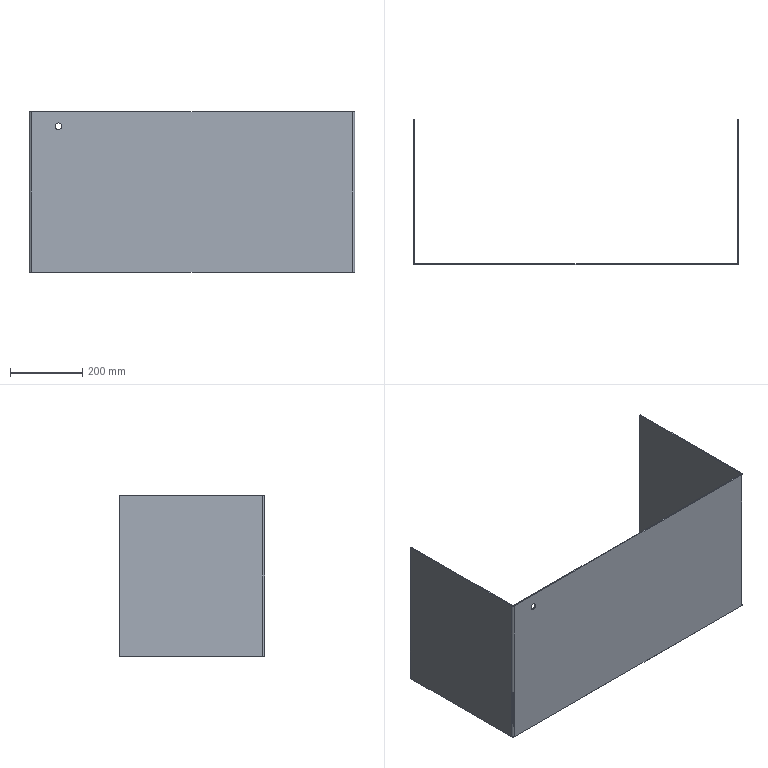Part | SolidWorks | features ICE 2, FlatPattern 1, SMBaseFlange 1, SheetMetal 1 | 1 solid | 28 faces | box 900 x 403 x 444 mm | volume 2258443 mm3 | plane 18 | cylinder 10 | commonest cylinder face diameters 7 x4 6 x2 12 x2 18.2 x2
STEP:
#1=CARTESIAN_POINT('',(80.,-403.,394.9));
#2=VERTEX_POINT('',#1);
#3=CARTESIAN_POINT('',(80.,-403.,413.1));
#4=VERTEX_POINT('',#3);
#5=CARTESIAN_POINT('',(80.,-403.,404.));
#6=DIRECTION('',(0.,1.,0.));
#7=DIRECTION('',(0.,0.,1.));
#8=AXIS2_PLACEMENT_3D('',#5,#6,#7);
#9=CIRCLE('',#8,9.1);
#10=EDGE_CURVE('',#2,#4,#9,.T.);
#11=ORIENTED_EDGE('',*,*,#10,.F.);
#12=CARTESIAN_POINT('',(80.,-400.,394.9));
#13=VERTEX_POINT('',#12);
#14=CARTESIAN_POINT('',(80.,-410.,394.9));
#15=DIRECTION('',(0.,1.,0.));
#16=VECTOR('',#15,1000.);
#17=LINE('',#14,#16);
#18=EDGE_CURVE('',#2,#13,#17,.T.);
#19=ORIENTED_EDGE('',*,*,#18,.T.);
#20=CARTESIAN_POINT('',(80.,-400.,413.1));
#21=VERTEX_POINT('',#20);
#22=CARTESIAN_POINT('',(80.,-400.,404.));
#23=DIRECTION('',(0.,1.,0.));
#24=DIRECTION('',(0.,0.,1.));
#25=AXIS2_PLACEMENT_3D('',#22,#23,#24);
#26=CIRCLE('',#25,9.1);
#27=EDGE_CURVE('',#13,#21,#26,.T.);
#28=ORIENTED_EDGE('',*,*,#27,.T.);
#29=CARTESIAN_POINT('',(80.,-410.,413.1));
#30=DIRECTION('',(0.,1.,0.));
#31=VECTOR('',#30,1000.);
#32=LINE('',#29,#31);
#33=EDGE_CURVE('',#4,#21,#32,.T.);
#34=ORIENTED_EDGE('',*,*,#33,.F.);
#35=EDGE_LOOP('',(#11,#19,#28,#34));
#36=FACE_OUTER_BOUND('',#35,.T.);
#37=CARTESIAN_POINT('',(80.,-410.,404.));
#38=DIRECTION('',(0.,1.,0.));
#39=DIRECTION('',(0.,0.,1.));
#40=AXIS2_PLACEMENT_3D('',#37,#38,#39);
#41=CYLINDRICAL_SURFACE('',#40,9.1);
#42=ADVANCED_FACE('',(#36),#41,.F.);
#43=CARTESIAN_POINT('',(900.,-3.5,0.));
#44=VERTEX_POINT('',#43);
#45=CARTESIAN_POINT('',(900.,0.,3.5));
#46=VERTEX_POINT('',#45);
#47=CARTESIAN_POINT('',(900.,-3.5,3.5));
#48=DIRECTION('',(1.,0.,0.));
#49=DIRECTION('',(0.,0.,1.));
#50=AXIS2_PLACEMENT_3D('',#47,#48,#49);
#51=CIRCLE('',#50,3.5);
#52=EDGE_CURVE('',#44,#46,#51,.T.);
#53=ORIENTED_EDGE('',*,*,#52,.T.);
#54=CARTESIAN_POINT('',(900.,0.,440.5));
#55=VERTEX_POINT('',#54);
#56=CARTESIAN_POINT('',(900.,0.,444.));
#57=DIRECTION('',(0.,0.,-1.));
#58=VECTOR('',#57,1000.);
#59=LINE('',#56,#58);
#60=EDGE_CURVE('',#55,#46,#59,.T.);
#61=ORIENTED_EDGE('',*,*,#60,.F.);
#62=CARTESIAN_POINT('',(900.,-3.5,444.));
#63=VERTEX_POINT('',#62);
#64=CARTESIAN_POINT('',(900.,-3.5,440.5));
#65=DIRECTION('',(1.,0.,0.));
#66=DIRECTION('',(0.,0.,1.));
#67=AXIS2_PLACEMENT_3D('',#64,#65,#66);
#68=CIRCLE('',#67,3.5);
#69=EDGE_CURVE('',#55,#63,#68,.T.);
#70=ORIENTED_EDGE('',*,*,#69,.T.);
#71=CARTESIAN_POINT('',(900.,-397.,444.));
#72=VERTEX_POINT('',#71);
#73=CARTESIAN_POINT('',(900.,-403.,444.));
#74=DIRECTION('',(0.,1.,0.));
#75=VECTOR('',#74,1000.);
#76=LINE('',#73,#75);
#77=EDGE_CURVE('',#72,#63,#76,.T.);
#78=ORIENTED_EDGE('',*,*,#77,.F.);
#79=CARTESIAN_POINT('',(900.,-397.,0.));
#80=VERTEX_POINT('',#79);
#81=CARTESIAN_POINT('',(900.,-397.,444.));
#82=DIRECTION('',(0.,0.,-1.));
#83=VECTOR('',#82,1000.);
#84=LINE('',#81,#83);
#85=EDGE_CURVE('',#72,#80,#84,.T.);
#86=ORIENTED_EDGE('',*,*,#85,.T.);
#87=CARTESIAN_POINT('',(900.,-403.,0.));
#88=DIRECTION('',(0.,1.,0.));
#89=VECTOR('',#88,1000.);
#90=LINE('',#87,#89);
#91=EDGE_CURVE('',#80,#44,#90,.T.);
#92=ORIENTED_EDGE('',*,*,#91,.T.);
#93=EDGE_LOOP('',(#53,#61,#70,#78,#86,#92));
#94=FACE_OUTER_BOUND('',#93,.T.);
#95=CARTESIAN_POINT('',(900.,-403.,444.));
#96=DIRECTION('',(-1.,0.,0.));
#97=DIRECTION('',(0.,0.,1.));
#98=AXIS2_PLACEMENT_3D('',#95,#96,#97);
#99=PLANE('',#98);
#100=ADVANCED_FACE('',(#94),#99,.F.);
#101=CARTESIAN_POINT('',(897.,0.,440.5));
#102=VERTEX_POINT('',#101);
#103=CARTESIAN_POINT('',(897.,0.,3.5));
#104=VERTEX_POINT('',#103);
#105=CARTESIAN_POINT('',(897.,0.,444.));
#106=DIRECTION('',(0.,0.,-1.));
#107=VECTOR('',#106,1000.);
#108=LINE('',#105,#107);
#109=EDGE_CURVE('',#102,#104,#108,.T.);
#110=ORIENTED_EDGE('',*,*,#109,.T.);
#111=CARTESIAN_POINT('',(897.,-3.5,0.));
#112=VERTEX_POINT('',#111);
#113=CARTESIAN_POINT('',(897.,-3.5,3.5));
#114=DIRECTION('',(1.,0.,0.));
#115=DIRECTION('',(0.,0.,1.));
#116=AXIS2_PLACEMENT_3D('',#113,#114,#115);
#117=CIRCLE('',#116,3.5);
#118=EDGE_CURVE('',#112,#104,#117,.T.);
#119=ORIENTED_EDGE('',*,*,#118,.F.);
#120=CARTESIAN_POINT('',(897.,-397.,0.));
#121=VERTEX_POINT('',#120);
#122=CARTESIAN_POINT('',(897.,-403.,0.));
#123=DIRECTION('',(0.,1.,0.));
#124=VECTOR('',#123,1000.);
#125=LINE('',#122,#124);
#126=EDGE_CURVE('',#121,#112,#125,.T.);
#127=ORIENTED_EDGE('',*,*,#126,.F.);
#128=CARTESIAN_POINT('',(897.,-397.,444.));
#129=VERTEX_POINT('',#128);
#130=CARTESIAN_POINT('',(897.,-397.,444.));
#131=DIRECTION('',(0.,0.,-1.));
#132=VECTOR('',#131,1000.);
#133=LINE('',#130,#132);
#134=EDGE_CURVE('',#129,#121,#133,.T.);
#135=ORIENTED_EDGE('',*,*,#134,.F.);
#136=CARTESIAN_POINT('',(897.,-3.5,444.));
#137=VERTEX_POINT('',#136);
#138=CARTESIAN_POINT('',(897.,-403.,444.));
#139=DIRECTION('',(0.,1.,0.));
#140=VECTOR('',#139,1000.);
#141=LINE('',#138,#140);
#142=EDGE_CURVE('',#129,#137,#141,.T.);
#143=ORIENTED_EDGE('',*,*,#142,.T.);
#144=CARTESIAN_POINT('',(897.,-3.5,440.5));
#145=DIRECTION('',(1.,0.,0.));
#146=DIRECTION('',(0.,0.,1.));
#147=AXIS2_PLACEMENT_3D('',#144,#145,#146);
#148=CIRCLE('',#147,3.5);
#149=EDGE_CURVE('',#102,#137,#148,.T.);
#150=ORIENTED_EDGE('',*,*,#149,.F.);
#151=EDGE_LOOP('',(#110,#119,#127,#135,#143,#150));
#152=FACE_OUTER_BOUND('',#151,.T.);
#153=CARTESIAN_POINT('',(897.,-403.,444.));
#154=DIRECTION('',(-1.,0.,0.));
#155=DIRECTION('',(0.,0.,1.));
#156=AXIS2_PLACEMENT_3D('',#153,#154,#155);
#157=PLANE('',#156);
#158=ADVANCED_FACE('',(#152),#157,.T.);
#159=ORIENTED_EDGE('',*,*,#60,.T.);
#160=CARTESIAN_POINT('',(897.,0.,3.5));
#161=DIRECTION('',(1.,0.,0.));
#162=VECTOR('',#161,1000.);
#163=LINE('',#160,#162);
#164=EDGE_CURVE('',#104,#46,#163,.T.);
#165=ORIENTED_EDGE('',*,*,#164,.F.);
#166=ORIENTED_EDGE('',*,*,#109,.F.);
#167=CARTESIAN_POINT('',(897.,0.,440.5));
#168=DIRECTION('',(1.,0.,0.));
#169=VECTOR('',#168,1000.);
#170=LINE('',#167,#169);
#171=EDGE_CURVE('',#102,#55,#170,.T.);
#172=ORIENTED_EDGE('',*,*,#171,.T.);
#173=EDGE_LOOP('',(#159,#165,#166,#172));
#174=FACE_OUTER_BOUND('',#173,.T.);
#175=CARTESIAN_POINT('',(897.,0.,444.));
#176=DIRECTION('',(0.,1.,0.));
#177=DIRECTION('',(0.,0.,1.));
#178=AXIS2_PLACEMENT_3D('',#175,#176,#177);
#179=PLANE('',#178);
#180=ADVANCED_FACE('',(#174),#179,.T.);
#181=CARTESIAN_POINT('',(3.,-3.5,0.));
#182=VERTEX_POINT('',#181);
#183=CARTESIAN_POINT('',(3.,-397.,0.));
#184=VERTEX_POINT('',#183);
#185=CARTESIAN_POINT('',(3.,0.,0.));
#186=DIRECTION('',(0.,-1.,0.));
#187=VECTOR('',#186,1000.);
#188=LINE('',#185,#187);
#189=EDGE_CURVE('',#182,#184,#188,.T.);
#190=ORIENTED_EDGE('',*,*,#189,.F.);
#191=CARTESIAN_POINT('',(3.,0.,3.5));
#192=VERTEX_POINT('',#191);
#193=CARTESIAN_POINT('',(3.,-3.5,3.5));
#194=DIRECTION('',(-1.,0.,0.));
#195=DIRECTION('',(0.,1.,0.));
#196=AXIS2_PLACEMENT_3D('',#193,#194,#195);
#197=CIRCLE('',#196,3.5);
#198=EDGE_CURVE('',#192,#182,#197,.T.);
#199=ORIENTED_EDGE('',*,*,#198,.F.);
#200=CARTESIAN_POINT('',(3.,0.,440.5));
#201=VERTEX_POINT('',#200);
#202=CARTESIAN_POINT('',(3.,0.,444.));
#203=DIRECTION('',(0.,0.,-1.));
#204=VECTOR('',#203,1000.);
#205=LINE('',#202,#204);
#206=EDGE_CURVE('',#201,#192,#205,.T.);
#207=ORIENTED_EDGE('',*,*,#206,.F.);
#208=CARTESIAN_POINT('',(3.,-3.5,444.));
#209=VERTEX_POINT('',#208);
#210=CARTESIAN_POINT('',(3.,-3.5,440.5));
#211=DIRECTION('',(-1.,0.,0.));
#212=DIRECTION('',(0.,1.,0.));
#213=AXIS2_PLACEMENT_3D('',#210,#211,#212);
#214=CIRCLE('',#213,3.5);
#215=EDGE_CURVE('',#209,#201,#214,.T.);
#216=ORIENTED_EDGE('',*,*,#215,.F.);
#217=CARTESIAN_POINT('',(3.,-397.,444.));
#218=VERTEX_POINT('',#217);
#219=CARTESIAN_POINT('',(3.,0.,444.));
#220=DIRECTION('',(0.,-1.,0.));
#221=VECTOR('',#220,1000.);
#222=LINE('',#219,#221);
#223=EDGE_CURVE('',#209,#218,#222,.T.);
#224=ORIENTED_EDGE('',*,*,#223,.T.);
#225=CARTESIAN_POINT('',(3.,-397.,444.));
#226=DIRECTION('',(0.,0.,-1.));
#227=VECTOR('',#226,1000.);
#228=LINE('',#225,#227);
#229=EDGE_CURVE('',#218,#184,#228,.T.);
#230=ORIENTED_EDGE('',*,*,#229,.T.);
#231=EDGE_LOOP('',(#190,#199,#207,#216,#224,#230));
#232=FACE_OUTER_BOUND('',#231,.T.);
#233=CARTESIAN_POINT('',(3.,0.,444.));
#234=DIRECTION('',(1.,0.,0.));
#235=DIRECTION('',(0.,1.,0.));
#236=AXIS2_PLACEMENT_3D('',#233,#234,#235);
#237=PLANE('',#236);
#238=ADVANCED_FACE('',(#232),#237,.T.);
#239=CARTESIAN_POINT('',(0.,0.,3.5));
#240=VERTEX_POINT('',#239);
#241=CARTESIAN_POINT('',(0.,-3.5,0.));
#242=VERTEX_POINT('',#241);
#243=CARTESIAN_POINT('',(0.,-3.5,3.5));
#244=DIRECTION('',(-1.,0.,0.));
#245=DIRECTION('',(0.,1.,0.));
#246=AXIS2_PLACEMENT_3D('',#243,#244,#245);
#247=CIRCLE('',#246,3.5);
#248=EDGE_CURVE('',#240,#242,#247,.T.);
#249=ORIENTED_EDGE('',*,*,#248,.T.);
#250=CARTESIAN_POINT('',(0.,-397.,0.));
#251=VERTEX_POINT('',#250);
#252=CARTESIAN_POINT('',(0.,0.,0.));
#253=DIRECTION('',(0.,-1.,0.));
#254=VECTOR('',#253,1000.);
#255=LINE('',#252,#254);
#256=EDGE_CURVE('',#242,#251,#255,.T.);
#257=ORIENTED_EDGE('',*,*,#256,.T.);
#258=CARTESIAN_POINT('',(0.,-397.,444.));
#259=VERTEX_POINT('',#258);
#260=CARTESIAN_POINT('',(0.,-397.,444.));
#261=DIRECTION('',(0.,0.,-1.));
#262=VECTOR('',#261,1000.);
#263=LINE('',#260,#262);
#264=EDGE_CURVE('',#259,#251,#263,.T.);
#265=ORIENTED_EDGE('',*,*,#264,.F.);
#266=CARTESIAN_POINT('',(0.,-3.5,444.));
#267=VERTEX_POINT('',#266);
#268=CARTESIAN_POINT('',(0.,0.,444.));
#269=DIRECTION('',(0.,-1.,0.));
#270=VECTOR('',#269,1000.);
#271=LINE('',#268,#270);
#272=EDGE_CURVE('',#267,#259,#271,.T.);
#273=ORIENTED_EDGE('',*,*,#272,.F.);
#274=CARTESIAN_POINT('',(0.,0.,440.5));
#275=VERTEX_POINT('',#274);
#276=CARTESIAN_POINT('',(0.,-3.5,440.5));
#277=DIRECTION('',(-1.,0.,0.));
#278=DIRECTION('',(0.,1.,0.));
#279=AXIS2_PLACEMENT_3D('',#276,#277,#278);
#280=CIRCLE('',#279,3.5);
#281=EDGE_CURVE('',#267,#275,#280,.T.);
#282=ORIENTED_EDGE('',*,*,#281,.T.);
#283=CARTESIAN_POINT('',(0.,0.,444.));
#284=DIRECTION('',(0.,0.,-1.));
#285=VECTOR('',#284,1000.);
#286=LINE('',#283,#285);
#287=EDGE_CURVE('',#275,#240,#286,.T.);
#288=ORIENTED_EDGE('',*,*,#287,.T.);
#289=EDGE_LOOP('',(#249,#257,#265,#273,#282,#288));
#290=FACE_OUTER_BOUND('',#289,.T.);
#291=CARTESIAN_POINT('',(0.,0.,444.));
#292=DIRECTION('',(1.,0.,0.));
#293=DIRECTION('',(0.,1.,0.));
#294=AXIS2_PLACEMENT_3D('',#291,#292,#293);
#295=PLANE('',#294);
#296=ADVANCED_FACE('',(#290),#295,.F.);
#297=ORIENTED_EDGE('',*,*,#77,.T.);
#298=CARTESIAN_POINT('',(897.,-3.5,444.));
#299=DIRECTION('',(1.,0.,0.));
#300=VECTOR('',#299,1000.);
#301=LINE('',#298,#300);
#302=EDGE_CURVE('',#137,#63,#301,.T.);
#303=ORIENTED_EDGE('',*,*,#302,.F.);
#304=ORIENTED_EDGE('',*,*,#142,.F.);
#305=CARTESIAN_POINT('',(897.,-397.,444.));
#306=DIRECTION('',(1.,0.,0.));
#307=VECTOR('',#306,1000.);
#308=LINE('',#305,#307);
#309=EDGE_CURVE('',#129,#72,#308,.T.);
#310=ORIENTED_EDGE('',*,*,#309,.T.);
#311=EDGE_LOOP('',(#297,#303,#304,#310));
#312=FACE_OUTER_BOUND('',#311,.T.);
#313=CARTESIAN_POINT('',(894.,-397.,444.));
#314=DIRECTION('',(0.,0.,1.));
#315=DIRECTION('',(1.,0.,0.));
#316=AXIS2_PLACEMENT_3D('',#313,#314,#315);
#317=PLANE('',#316);
#318=ADVANCED_FACE('',(#312),#317,.T.);
#319=CARTESIAN_POINT('',(3.,0.,3.5));
#320=DIRECTION('',(-1.,0.,0.));
#321=VECTOR('',#320,1000.);
#322=LINE('',#319,#321);
#323=EDGE_CURVE('',#192,#240,#322,.T.);
#324=ORIENTED_EDGE('',*,*,#323,.T.);
#325=ORIENTED_EDGE('',*,*,#287,.F.);
#326=CARTESIAN_POINT('',(3.,0.,440.5));
#327=DIRECTION('',(-1.,0.,0.));
#328=VECTOR('',#327,1000.);
#329=LINE('',#326,#328);
#330=EDGE_CURVE('',#201,#275,#329,.T.);
#331=ORIENTED_EDGE('',*,*,#330,.F.);
#332=ORIENTED_EDGE('',*,*,#206,.T.);
#333=EDGE_LOOP('',(#324,#325,#331,#332));
#334=FACE_OUTER_BOUND('',#333,.T.);
#335=CARTESIAN_POINT('',(0.,0.,444.));
#336=DIRECTION('',(0.,1.,0.));
#337=DIRECTION('',(-1.,0.,0.));
#338=AXIS2_PLACEMENT_3D('',#335,#336,#337);
#339=PLANE('',#338);
#340=ADVANCED_FACE('',(#334),#339,.T.);
#341=CARTESIAN_POINT('',(0.,-397.,444.));
#342=DIRECTION('',(1.,0.,0.));
#343=VECTOR('',#342,1000.);
#344=LINE('',#341,#343);
#345=EDGE_CURVE('',#259,#218,#344,.T.);
#346=ORIENTED_EDGE('',*,*,#345,.F.);
#347=CARTESIAN_POINT('',(6.,-403.,444.));
#348=VERTEX_POINT('',#347);
#349=CARTESIAN_POINT('',(6.,-397.,444.));
#350=DIRECTION('',(0.,0.,1.));
#351=DIRECTION('',(-1.,0.,0.));
#352=AXIS2_PLACEMENT_3D('',#349,#350,#351);
#353=CIRCLE('',#352,6.);
#354=EDGE_CURVE('',#259,#348,#353,.T.);
#355=ORIENTED_EDGE('',*,*,#354,.T.);
#356=CARTESIAN_POINT('',(6.,-400.,444.));
#357=VERTEX_POINT('',#356);
#358=CARTESIAN_POINT('',(6.,-400.,444.));
#359=DIRECTION('',(0.,-1.,0.));
#360=VECTOR('',#359,1000.);
#361=LINE('',#358,#360);
#362=EDGE_CURVE('',#357,#348,#361,.T.);
#363=ORIENTED_EDGE('',*,*,#362,.F.);
#364=CARTESIAN_POINT('',(6.,-397.,444.));
#365=DIRECTION('',(0.,0.,1.));
#366=DIRECTION('',(1.,0.,0.));
#367=AXIS2_PLACEMENT_3D('',#364,#365,#366);
#368=CIRCLE('',#367,3.);
#369=EDGE_CURVE('',#218,#357,#368,.T.);
#370=ORIENTED_EDGE('',*,*,#369,.F.);
#371=EDGE_LOOP('',(#346,#355,#363,#370));
#372=FACE_OUTER_BOUND('',#371,.T.);
#373=CARTESIAN_POINT('',(0.,-397.,444.));
#374=DIRECTION('',(0.,0.,1.));
#375=DIRECTION('',(1.,0.,0.));
#376=AXIS2_PLACEMENT_3D('',#373,#374,#375);
#377=PLANE('',#376);
#378=ADVANCED_FACE('',(#372),#377,.T.);
#379=CARTESIAN_POINT('',(3.,-3.5,444.));
#380=DIRECTION('',(-1.,0.,0.));
#381=VECTOR('',#380,1000.);
#382=LINE('',#379,#381);
#383=EDGE_CURVE('',#209,#267,#382,.T.);
#384=ORIENTED_EDGE('',*,*,#383,.T.);
#385=ORIENTED_EDGE('',*,*,#272,.T.);
#386=ORIENTED_EDGE('',*,*,#345,.T.);
#387=ORIENTED_EDGE('',*,*,#223,.F.);
#388=EDGE_LOOP('',(#384,#385,#386,#387));
#389=FACE_OUTER_BOUND('',#388,.T.);
#390=CARTESIAN_POINT('',(6.,-400.,444.));
#391=DIRECTION('',(0.,0.,1.));
#392=DIRECTION('',(1.,0.,0.));
#393=AXIS2_PLACEMENT_3D('',#390,#391,#392);
#394=PLANE('',#393);
#395=ADVANCED_FACE('',(#389),#394,.T.);
#396=CARTESIAN_POINT('',(6.,-403.,0.));
#397=VERTEX_POINT('',#396);
#398=CARTESIAN_POINT('',(6.,-400.,0.));
#399=VERTEX_POINT('',#398);
#400=CARTESIAN_POINT('',(6.,-403.,0.));
#401=DIRECTION('',(0.,1.,0.));
#402=VECTOR('',#401,1000.);
#403=LINE('',#400,#402);
#404=EDGE_CURVE('',#397,#399,#403,.T.);
#405=ORIENTED_EDGE('',*,*,#404,.F.);
#406=CARTESIAN_POINT('',(6.,-397.,0.));
#407=DIRECTION('',(0.,0.,1.));
#408=DIRECTION('',(-1.,0.,0.));
#409=AXIS2_PLACEMENT_3D('',#406,#407,#408);
#410=CIRCLE('',#409,6.);
#411=EDGE_CURVE('',#251,#397,#410,.T.);
#412=ORIENTED_EDGE('',*,*,#411,.F.);
#413=CARTESIAN_POINT('',(3.,-397.,0.));
#414=DIRECTION('',(-1.,0.,0.));
#415=VECTOR('',#414,1000.);
#416=LINE('',#413,#415);
#417=EDGE_CURVE('',#184,#251,#416,.T.);
#418=ORIENTED_EDGE('',*,*,#417,.F.);
#419=CARTESIAN_POINT('',(6.,-397.,0.));
#420=DIRECTION('',(0.,0.,1.));
#421=DIRECTION('',(1.,0.,0.));
#422=AXIS2_PLACEMENT_3D('',#419,#420,#421);
#423=CIRCLE('',#422,3.);
#424=EDGE_CURVE('',#184,#399,#423,.T.);
#425=ORIENTED_EDGE('',*,*,#424,.T.);
#426=EDGE_LOOP('',(#405,#412,#418,#425));
#427=FACE_OUTER_BOUND('',#426,.T.);
#428=CARTESIAN_POINT('',(6.,-403.,0.));
#429=DIRECTION('',(0.,0.,-1.));
#430=DIRECTION('',(-1.,0.,0.));
#431=AXIS2_PLACEMENT_3D('',#428,#429,#430);
#432=PLANE('',#431);
#433=ADVANCED_FACE('',(#427),#432,.T.);
#434=CARTESIAN_POINT('',(894.,-403.,0.));
#435=VERTEX_POINT('',#434);
#436=CARTESIAN_POINT('',(0.,-403.,0.));
#437=DIRECTION('',(1.,0.,0.));
#438=VECTOR('',#437,1000.);
#439=LINE('',#436,#438);
#440=EDGE_CURVE('',#397,#435,#439,.T.);
#441=ORIENTED_EDGE('',*,*,#440,.F.);
#442=ORIENTED_EDGE('',*,*,#404,.T.);
#443=CARTESIAN_POINT('',(894.,-400.,0.));
#444=VERTEX_POINT('',#443);
#445=CARTESIAN_POINT('',(0.,-400.,0.));
#446=DIRECTION('',(1.,0.,0.));
#447=VECTOR('',#446,1000.);
#448=LINE('',#445,#447);
#449=EDGE_CURVE('',#399,#444,#448,.T.);
#450=ORIENTED_EDGE('',*,*,#449,.T.);
#451=CARTESIAN_POINT('',(894.,-400.,0.));
#452=DIRECTION('',(0.,-1.,0.));
#453=VECTOR('',#452,1000.);
#454=LINE('',#451,#453);
#455=EDGE_CURVE('',#444,#435,#454,.T.);
#456=ORIENTED_EDGE('',*,*,#455,.T.);
#457=EDGE_LOOP('',(#441,#442,#450,#456));
#458=FACE_OUTER_BOUND('',#457,.T.);
#459=CARTESIAN_POINT('',(3.,-397.,0.));
#460=DIRECTION('',(0.,0.,-1.));
#461=DIRECTION('',(-1.,0.,0.));
#462=AXIS2_PLACEMENT_3D('',#459,#460,#461);
#463=PLANE('',#462);
#464=ADVANCED_FACE('',(#458),#463,.T.);
#465=CARTESIAN_POINT('',(894.,-403.,444.));
#466=VERTEX_POINT('',#465);
#467=CARTESIAN_POINT('',(894.,-400.,444.));
#468=VERTEX_POINT('',#467);
#469=CARTESIAN_POINT('',(894.,-403.,444.));
#470=DIRECTION('',(0.,1.,0.));
#471=VECTOR('',#470,1000.);
#472=LINE('',#469,#471);
#473=EDGE_CURVE('',#466,#468,#472,.T.);
#474=ORIENTED_EDGE('',*,*,#473,.F.);
#475=CARTESIAN_POINT('',(894.,-397.,444.));
#476=DIRECTION('',(0.,0.,1.));
#477=DIRECTION('',(-1.,0.,0.));
#478=AXIS2_PLACEMENT_3D('',#475,#476,#477);
#479=CIRCLE('',#478,6.);
#480=EDGE_CURVE('',#466,#72,#479,.T.);
#481=ORIENTED_EDGE('',*,*,#480,.T.);
#482=ORIENTED_EDGE('',*,*,#309,.F.);
#483=CARTESIAN_POINT('',(894.,-397.,444.));
#484=DIRECTION('',(0.,0.,1.));
#485=DIRECTION('',(1.,0.,0.));
#486=AXIS2_PLACEMENT_3D('',#483,#484,#485);
#487=CIRCLE('',#486,3.);
#488=EDGE_CURVE('',#468,#129,#487,.T.);
#489=ORIENTED_EDGE('',*,*,#488,.F.);
#490=EDGE_LOOP('',(#474,#481,#482,#489));
#491=FACE_OUTER_BOUND('',#490,.T.);
#492=CARTESIAN_POINT('',(894.,-403.,444.));
#493=DIRECTION('',(0.,0.,1.));
#494=DIRECTION('',(1.,0.,0.));
#495=AXIS2_PLACEMENT_3D('',#492,#493,#494);
#496=PLANE('',#495);
#497=ADVANCED_FACE('',(#491),#496,.T.);
#498=CARTESIAN_POINT('',(0.,-403.,444.));
#499=DIRECTION('',(1.,0.,0.));
#500=VECTOR('',#499,1000.);
#501=LINE('',#498,#500);
#502=EDGE_CURVE('',#348,#466,#501,.T.);
#503=ORIENTED_EDGE('',*,*,#502,.T.);
#504=ORIENTED_EDGE('',*,*,#473,.T.);
#505=CARTESIAN_POINT('',(0.,-400.,444.));
#506=DIRECTION('',(1.,0.,0.));
#507=VECTOR('',#506,1000.);
#508=LINE('',#505,#507);
#509=EDGE_CURVE('',#357,#468,#508,.T.);
#510=ORIENTED_EDGE('',*,*,#509,.F.);
#511=ORIENTED_EDGE('',*,*,#362,.T.);
#512=EDGE_LOOP('',(#503,#504,#510,#511));
#513=FACE_OUTER_BOUND('',#512,.T.);
#514=CARTESIAN_POINT('',(897.,-397.,444.));
#515=DIRECTION('',(0.,0.,1.));
#516=DIRECTION('',(1.,0.,0.));
#517=AXIS2_PLACEMENT_3D('',#514,#515,#516);
#518=PLANE('',#517);
#519=ADVANCED_FACE('',(#513),#518,.T.);
#520=CARTESIAN_POINT('',(900.,-397.,0.));
#521=DIRECTION('',(-1.,0.,0.));
#522=VECTOR('',#521,1000.);
#523=LINE('',#520,#522);
#524=EDGE_CURVE('',#80,#121,#523,.T.);
#525=ORIENTED_EDGE('',*,*,#524,.F.);
#526=CARTESIAN_POINT('',(894.,-397.,0.));
#527=DIRECTION('',(0.,0.,1.));
#528=DIRECTION('',(-1.,0.,0.));
#529=AXIS2_PLACEMENT_3D('',#526,#527,#528);
#530=CIRCLE('',#529,6.);
#531=EDGE_CURVE('',#435,#80,#530,.T.);
#532=ORIENTED_EDGE('',*,*,#531,.F.);
#533=ORIENTED_EDGE('',*,*,#455,.F.);
#534=CARTESIAN_POINT('',(894.,-397.,0.));
#535=DIRECTION('',(0.,0.,1.));
#536=DIRECTION('',(1.,0.,0.));
#537=AXIS2_PLACEMENT_3D('',#534,#535,#536);
#538=CIRCLE('',#537,3.);
#539=EDGE_CURVE('',#444,#121,#538,.T.);
#540=ORIENTED_EDGE('',*,*,#539,.T.);
#541=EDGE_LOOP('',(#525,#532,#533,#540));
#542=FACE_OUTER_BOUND('',#541,.T.);
#543=CARTESIAN_POINT('',(900.,-397.,0.));
#544=DIRECTION('',(0.,0.,-1.));
#545=DIRECTION('',(-1.,0.,0.));
#546=AXIS2_PLACEMENT_3D('',#543,#544,#545);
#547=PLANE('',#546);
#548=ADVANCED_FACE('',(#542),#547,.T.);
#549=CARTESIAN_POINT('',(897.,-3.5,0.));
#550=DIRECTION('',(1.,0.,0.));
#551=VECTOR('',#550,1000.);
#552=LINE('',#549,#551);
#553=EDGE_CURVE('',#112,#44,#552,.T.);
#554=ORIENTED_EDGE('',*,*,#553,.T.);
#555=ORIENTED_EDGE('',*,*,#91,.F.);
#556=ORIENTED_EDGE('',*,*,#524,.T.);
#557=ORIENTED_EDGE('',*,*,#126,.T.);
#558=EDGE_LOOP('',(#554,#555,#556,#557));
#559=FACE_OUTER_BOUND('',#558,.T.);
#560=CARTESIAN_POINT('',(894.,-400.,0.));
#561=DIRECTION('',(0.,0.,-1.));
#562=DIRECTION('',(-1.,0.,0.));
#563=AXIS2_PLACEMENT_3D('',#560,#561,#562);
#564=PLANE('',#563);
#565=ADVANCED_FACE('',(#559),#564,.T.);
#566=ORIENTED_EDGE('',*,*,#539,.F.);
#567=CARTESIAN_POINT('',(894.,-400.,444.));
#568=DIRECTION('',(0.,0.,-1.));
#569=VECTOR('',#568,1000.);
#570=LINE('',#567,#569);
#571=EDGE_CURVE('',#468,#444,#570,.T.);
#572=ORIENTED_EDGE('',*,*,#571,.F.);
#573=ORIENTED_EDGE('',*,*,#488,.T.);
#574=ORIENTED_EDGE('',*,*,#134,.T.);
#575=EDGE_LOOP('',(#566,#572,#573,#574));
#576=FACE_OUTER_BOUND('',#575,.T.);
#577=CARTESIAN_POINT('',(894.,-397.,444.));
#578=DIRECTION('',(0.,0.,-1.));
#579=DIRECTION('',(-1.,0.,0.));
#580=AXIS2_PLACEMENT_3D('',#577,#578,#579);
#581=CYLINDRICAL_SURFACE('',#580,3.);
#582=ADVANCED_FACE('',(#576),#581,.F.);
#583=CARTESIAN_POINT('',(80.,-400.,404.));
#584=DIRECTION('',(0.,1.,0.));
#585=DIRECTION('',(0.,0.,1.));
#586=AXIS2_PLACEMENT_3D('',#583,#584,#585);
#587=CIRCLE('',#586,9.1);
#588=EDGE_CURVE('',#21,#13,#587,.T.);
#589=ORIENTED_EDGE('',*,*,#588,.F.);
#590=ORIENTED_EDGE('',*,*,#27,.F.);
#591=EDGE_LOOP('',(#589,#590));
#592=FACE_BOUND('',#591,.T.);
#593=ORIENTED_EDGE('',*,*,#449,.F.);
#594=CARTESIAN_POINT('',(6.,-400.,444.));
#595=DIRECTION('',(0.,0.,-1.));
#596=VECTOR('',#595,1000.);
#597=LINE('',#594,#596);
#598=EDGE_CURVE('',#357,#399,#597,.T.);
#599=ORIENTED_EDGE('',*,*,#598,.F.);
#600=ORIENTED_EDGE('',*,*,#509,.T.);
#601=ORIENTED_EDGE('',*,*,#571,.T.);
#602=EDGE_LOOP('',(#593,#599,#600,#601));
#603=FACE_OUTER_BOUND('',#602,.T.);
#604=CARTESIAN_POINT('',(0.,-400.,444.));
#605=DIRECTION('',(0.,1.,0.));
#606=DIRECTION('',(0.,0.,1.));
#607=AXIS2_PLACEMENT_3D('',#604,#605,#606);
#608=PLANE('',#607);
#609=ADVANCED_FACE('',(#592,#603),#608,.T.);
#610=ORIENTED_EDGE('',*,*,#424,.F.);
#611=ORIENTED_EDGE('',*,*,#229,.F.);
#612=ORIENTED_EDGE('',*,*,#369,.T.);
#613=ORIENTED_EDGE('',*,*,#598,.T.);
#614=EDGE_LOOP('',(#610,#611,#612,#613));
#615=FACE_OUTER_BOUND('',#614,.T.);
#616=CARTESIAN_POINT('',(6.,-397.,444.));
#617=DIRECTION('',(0.,0.,-1.));
#618=DIRECTION('',(-1.,0.,0.));
#619=AXIS2_PLACEMENT_3D('',#616,#617,#618);
#620=CYLINDRICAL_SURFACE('',#619,3.);
#621=ADVANCED_FACE('',(#615),#620,.F.);
#622=ORIENTED_EDGE('',*,*,#411,.T.);
#623=CARTESIAN_POINT('',(6.,-403.,444.));
#624=DIRECTION('',(0.,0.,-1.));
#625=VECTOR('',#624,1000.);
#626=LINE('',#623,#625);
#627=EDGE_CURVE('',#348,#397,#626,.T.);
#628=ORIENTED_EDGE('',*,*,#627,.F.);
#629=ORIENTED_EDGE('',*,*,#354,.F.);
#630=ORIENTED_EDGE('',*,*,#264,.T.);
#631=EDGE_LOOP('',(#622,#628,#629,#630));
#632=FACE_OUTER_BOUND('',#631,.T.);
#633=CARTESIAN_POINT('',(6.,-397.,444.));
#634=DIRECTION('',(0.,0.,-1.));
#635=DIRECTION('',(-1.,0.,0.));
#636=AXIS2_PLACEMENT_3D('',#633,#634,#635);
#637=CYLINDRICAL_SURFACE('',#636,6.);
#638=ADVANCED_FACE('',(#632),#637,.T.);
#639=CARTESIAN_POINT('',(80.,-403.,404.));
#640=DIRECTION('',(0.,1.,0.));
#641=DIRECTION('',(0.,0.,1.));
#642=AXIS2_PLACEMENT_3D('',#639,#640,#641);
#643=CIRCLE('',#642,9.1);
#644=EDGE_CURVE('',#4,#2,#643,.T.);
#645=ORIENTED_EDGE('',*,*,#644,.T.);
#646=ORIENTED_EDGE('',*,*,#10,.T.);
#647=EDGE_LOOP('',(#645,#646));
#648=FACE_BOUND('',#647,.T.);
#649=ORIENTED_EDGE('',*,*,#440,.T.);
#650=CARTESIAN_POINT('',(894.,-403.,444.));
#651=DIRECTION('',(0.,0.,-1.));
#652=VECTOR('',#651,1000.);
#653=LINE('',#650,#652);
#654=EDGE_CURVE('',#466,#435,#653,.T.);
#655=ORIENTED_EDGE('',*,*,#654,.F.);
#656=ORIENTED_EDGE('',*,*,#502,.F.);
#657=ORIENTED_EDGE('',*,*,#627,.T.);
#658=EDGE_LOOP('',(#649,#655,#656,#657));
#659=FACE_OUTER_BOUND('',#658,.T.);
#660=CARTESIAN_POINT('',(0.,-403.,444.));
#661=DIRECTION('',(0.,1.,0.));
#662=DIRECTION('',(0.,0.,1.));
#663=AXIS2_PLACEMENT_3D('',#660,#661,#662);
#664=PLANE('',#663);
#665=ADVANCED_FACE('',(#648,#659),#664,.F.);
#666=ORIENTED_EDGE('',*,*,#531,.T.);
#667=ORIENTED_EDGE('',*,*,#85,.F.);
#668=ORIENTED_EDGE('',*,*,#480,.F.);
#669=ORIENTED_EDGE('',*,*,#654,.T.);
#670=EDGE_LOOP('',(#666,#667,#668,#669));
#671=FACE_OUTER_BOUND('',#670,.T.);
#672=CARTESIAN_POINT('',(894.,-397.,444.));
#673=DIRECTION('',(0.,0.,-1.));
#674=DIRECTION('',(-1.,0.,0.));
#675=AXIS2_PLACEMENT_3D('',#672,#673,#674);
#676=CYLINDRICAL_SURFACE('',#675,6.);
#677=ADVANCED_FACE('',(#671),#676,.T.);
#678=ORIENTED_EDGE('',*,*,#256,.F.);
#679=CARTESIAN_POINT('',(3.,-3.5,0.));
#680=DIRECTION('',(-1.,0.,0.));
#681=VECTOR('',#680,1000.);
#682=LINE('',#679,#681);
#683=EDGE_CURVE('',#182,#242,#682,.T.);
#684=ORIENTED_EDGE('',*,*,#683,.F.);
#685=ORIENTED_EDGE('',*,*,#189,.T.);
#686=ORIENTED_EDGE('',*,*,#417,.T.);
#687=EDGE_LOOP('',(#678,#684,#685,#686));
#688=FACE_OUTER_BOUND('',#687,.T.);
#689=CARTESIAN_POINT('',(894.,-397.,0.));
#690=DIRECTION('',(0.,0.,1.));
#691=DIRECTION('',(1.,0.,0.));
#692=AXIS2_PLACEMENT_3D('',#689,#690,#691);
#693=PLANE('',#692);
#694=ADVANCED_FACE('',(#688),#693,.F.);
#695=ORIENTED_EDGE('',*,*,#18,.F.);
#696=ORIENTED_EDGE('',*,*,#644,.F.);
#697=ORIENTED_EDGE('',*,*,#33,.T.);
#698=ORIENTED_EDGE('',*,*,#588,.T.);
#699=EDGE_LOOP('',(#695,#696,#697,#698));
#700=FACE_OUTER_BOUND('',#699,.T.);
#701=CARTESIAN_POINT('',(80.,-410.,404.));
#702=DIRECTION('',(0.,1.,0.));
#703=DIRECTION('',(0.,0.,1.));
#704=AXIS2_PLACEMENT_3D('',#701,#702,#703);
#705=CYLINDRICAL_SURFACE('',#704,9.1);
#706=ADVANCED_FACE('',(#700),#705,.F.);
#707=ORIENTED_EDGE('',*,*,#215,.T.);
#708=ORIENTED_EDGE('',*,*,#330,.T.);
#709=ORIENTED_EDGE('',*,*,#281,.F.);
#710=ORIENTED_EDGE('',*,*,#383,.F.);
#711=EDGE_LOOP('',(#707,#708,#709,#710));
#712=FACE_OUTER_BOUND('',#711,.T.);
#713=CARTESIAN_POINT('',(3.,-3.5,440.5));
#714=DIRECTION('',(1.,0.,0.));
#715=DIRECTION('',(0.,1.,0.));
#716=AXIS2_PLACEMENT_3D('',#713,#714,#715);
#717=CYLINDRICAL_SURFACE('',#716,3.5);
#718=ADVANCED_FACE('',(#712),#717,.T.);
#719=ORIENTED_EDGE('',*,*,#149,.T.);
#720=ORIENTED_EDGE('',*,*,#302,.T.);
#721=ORIENTED_EDGE('',*,*,#69,.F.);
#722=ORIENTED_EDGE('',*,*,#171,.F.);
#723=EDGE_LOOP('',(#719,#720,#721,#722));
#724=FACE_OUTER_BOUND('',#723,.T.);
#725=CARTESIAN_POINT('',(897.,-3.5,440.5));
#726=DIRECTION('',(-1.,0.,0.));
#727=DIRECTION('',(0.,0.,1.));
#728=AXIS2_PLACEMENT_3D('',#725,#726,#727);
#729=CYLINDRICAL_SURFACE('',#728,3.5);
#730=ADVANCED_FACE('',(#724),#729,.T.);
#731=ORIENTED_EDGE('',*,*,#198,.T.);
#732=ORIENTED_EDGE('',*,*,#683,.T.);
#733=ORIENTED_EDGE('',*,*,#248,.F.);
#734=ORIENTED_EDGE('',*,*,#323,.F.);
#735=EDGE_LOOP('',(#731,#732,#733,#734));
#736=FACE_OUTER_BOUND('',#735,.T.);
#737=CARTESIAN_POINT('',(3.,-3.5,3.5));
#738=DIRECTION('',(1.,0.,0.));
#739=DIRECTION('',(0.,1.,0.));
#740=AXIS2_PLACEMENT_3D('',#737,#738,#739);
#741=CYLINDRICAL_SURFACE('',#740,3.5);
#742=ADVANCED_FACE('',(#736),#741,.T.);
#743=ORIENTED_EDGE('',*,*,#118,.T.);
#744=ORIENTED_EDGE('',*,*,#164,.T.);
#745=ORIENTED_EDGE('',*,*,#52,.F.);
#746=ORIENTED_EDGE('',*,*,#553,.F.);
#747=EDGE_LOOP('',(#743,#744,#745,#746));
#748=FACE_OUTER_BOUND('',#747,.T.);
#749=CARTESIAN_POINT('',(897.,-3.5,3.5));
#750=DIRECTION('',(-1.,0.,0.));
#751=DIRECTION('',(0.,0.,1.));
#752=AXIS2_PLACEMENT_3D('',#749,#750,#751);
#753=CYLINDRICAL_SURFACE('',#752,3.5);
#754=ADVANCED_FACE('',(#748),#753,.T.);
#755=CLOSED_SHELL('',(#42,#100,#158,#180,#238,#296,#318,#340,#378,#395,#433,#464,#497,#519,#548,#565,#582,#609,#621,#638,#665,#677,#694,#706,#718,#730,#742,#754));
#756=MANIFOLD_SOLID_BREP('',#755);
#757=CARTESIAN_POINT('',(0.,0.,0.));
#758=DIRECTION('',(0.,0.,1.));
#759=DIRECTION('',(1.,0.,0.));
#760=AXIS2_PLACEMENT_3D('',#757,#758,#759);
#761=(LENGTH_UNIT()NAMED_UNIT(*)SI_UNIT(.MILLI.,.METRE.));
#762=UNCERTAINTY_MEASURE_WITH_UNIT(LENGTH_MEASURE(0.00001),#761,'','');
#763=(NAMED_UNIT(*)PLANE_ANGLE_UNIT()SI_UNIT($,.RADIAN.));
#764=(NAMED_UNIT(*)SI_UNIT($,.STERADIAN.)SOLID_ANGLE_UNIT());
#765=(GEOMETRIC_REPRESENTATION_CONTEXT(3)GLOBAL_UNCERTAINTY_ASSIGNED_CONTEXT((#762))GLOBAL_UNIT_ASSIGNED_CONTEXT((#761,#763,#764))REPRESENTATION_CONTEXT('',''));
#766=ADVANCED_BREP_SHAPE_REPRESENTATION('',(#756,#760),#765);